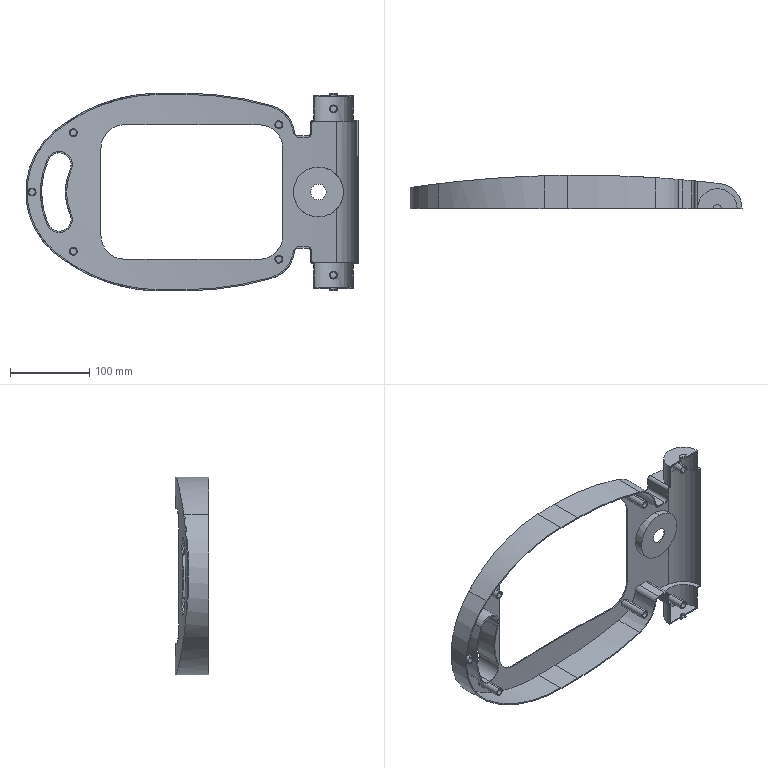Part | SolidWorks | features ICE 9, CombineBodies 1, Extrusion 1, Fillet 1, Shell 1 | 1 solid | 134 faces | box 420 x 41.94 x 250 mm | volume 152535 mm3 | cylinder 93 | plane 41 | commonest cylinder face diameters 8 x18 10 x18 60 x6 2997 x6 47 x4 30 x3